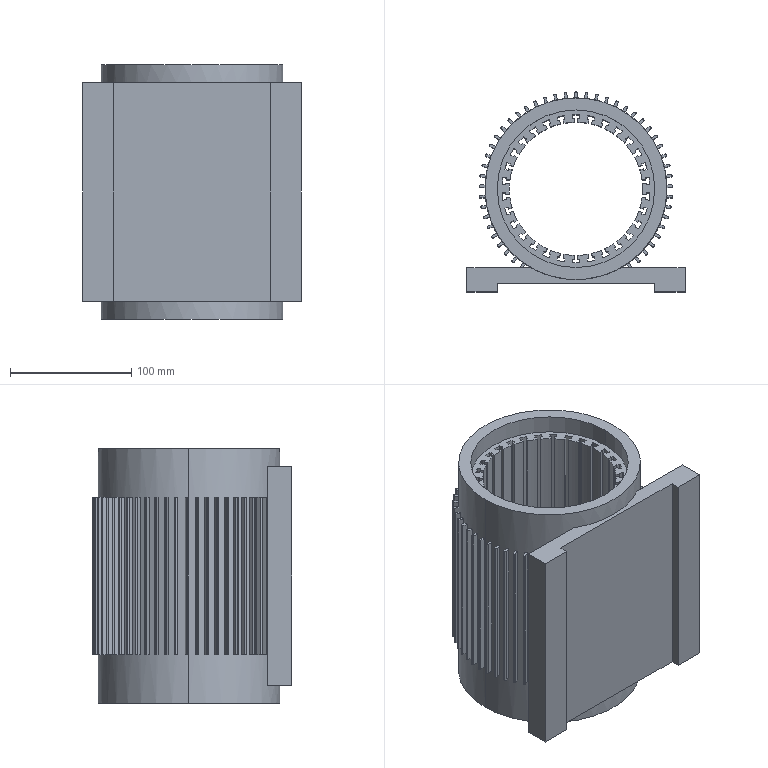Part | SolidWorks | 1 solid | 832 faces | box 180 x 165 x 210 mm | volume 1913564 mm3 | plane 458 | cylinder 374 | commonest cylinder face diameters 0.479 x222 2 x115 110 x31 130 x4 150 x2